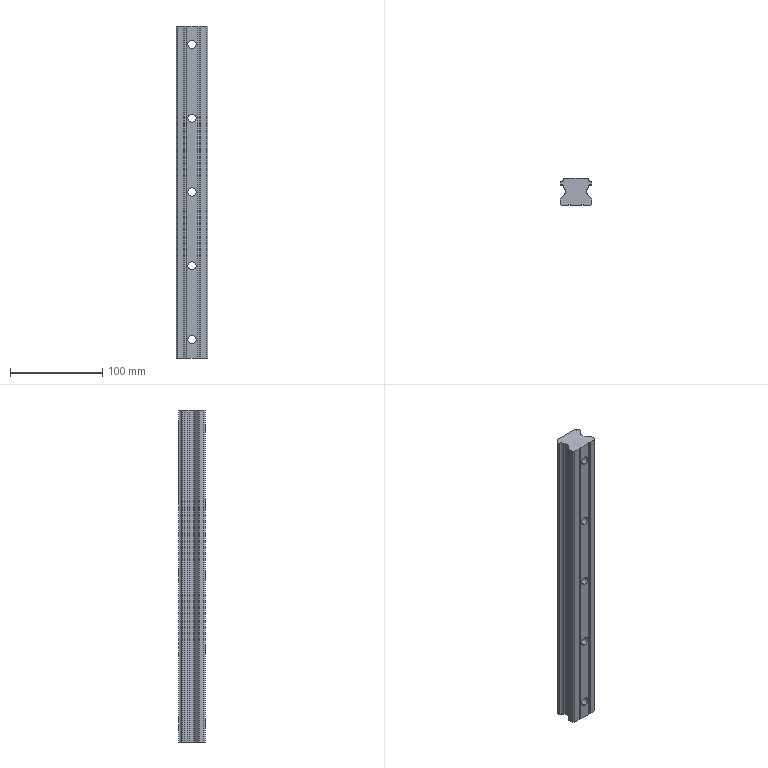Part | SolidWorks | features BaseBody 1, HoleWzd 1, ICE 1, LPattern 1 | 1 solid | 65 faces | box 34 x 29 x 360 mm | volume 291889 mm3 | plane 35 | cylinder 30 | commonest cylinder face diameters 9 x10 2.4 x6 14 x6 6.5 x4 15 x4